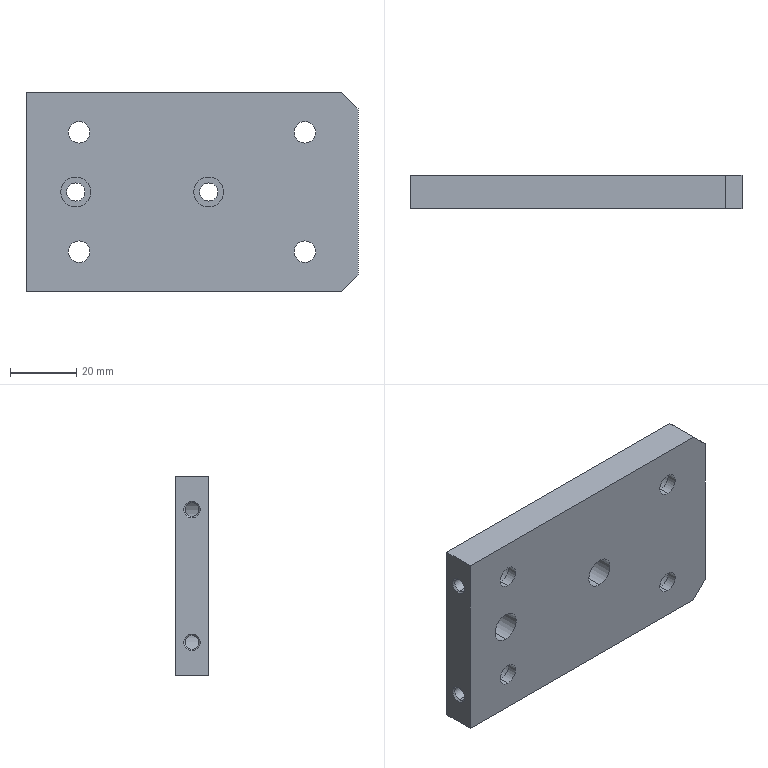Part | STEP file | B1-014 | 1 solid | 48 faces | box 100 x 10 x 60 mm | volume 55350 mm3 | cylinder 28 | plane 14 | cone 6 | commonest cylinder face diameters 6.5 x8 11 x8 4.2 x4 5.5 x4 9 x4